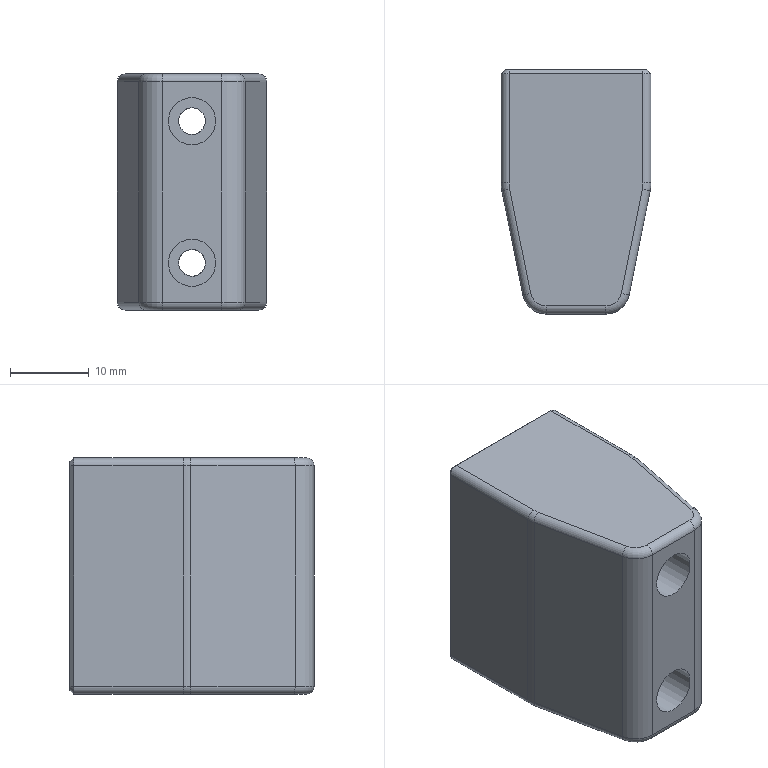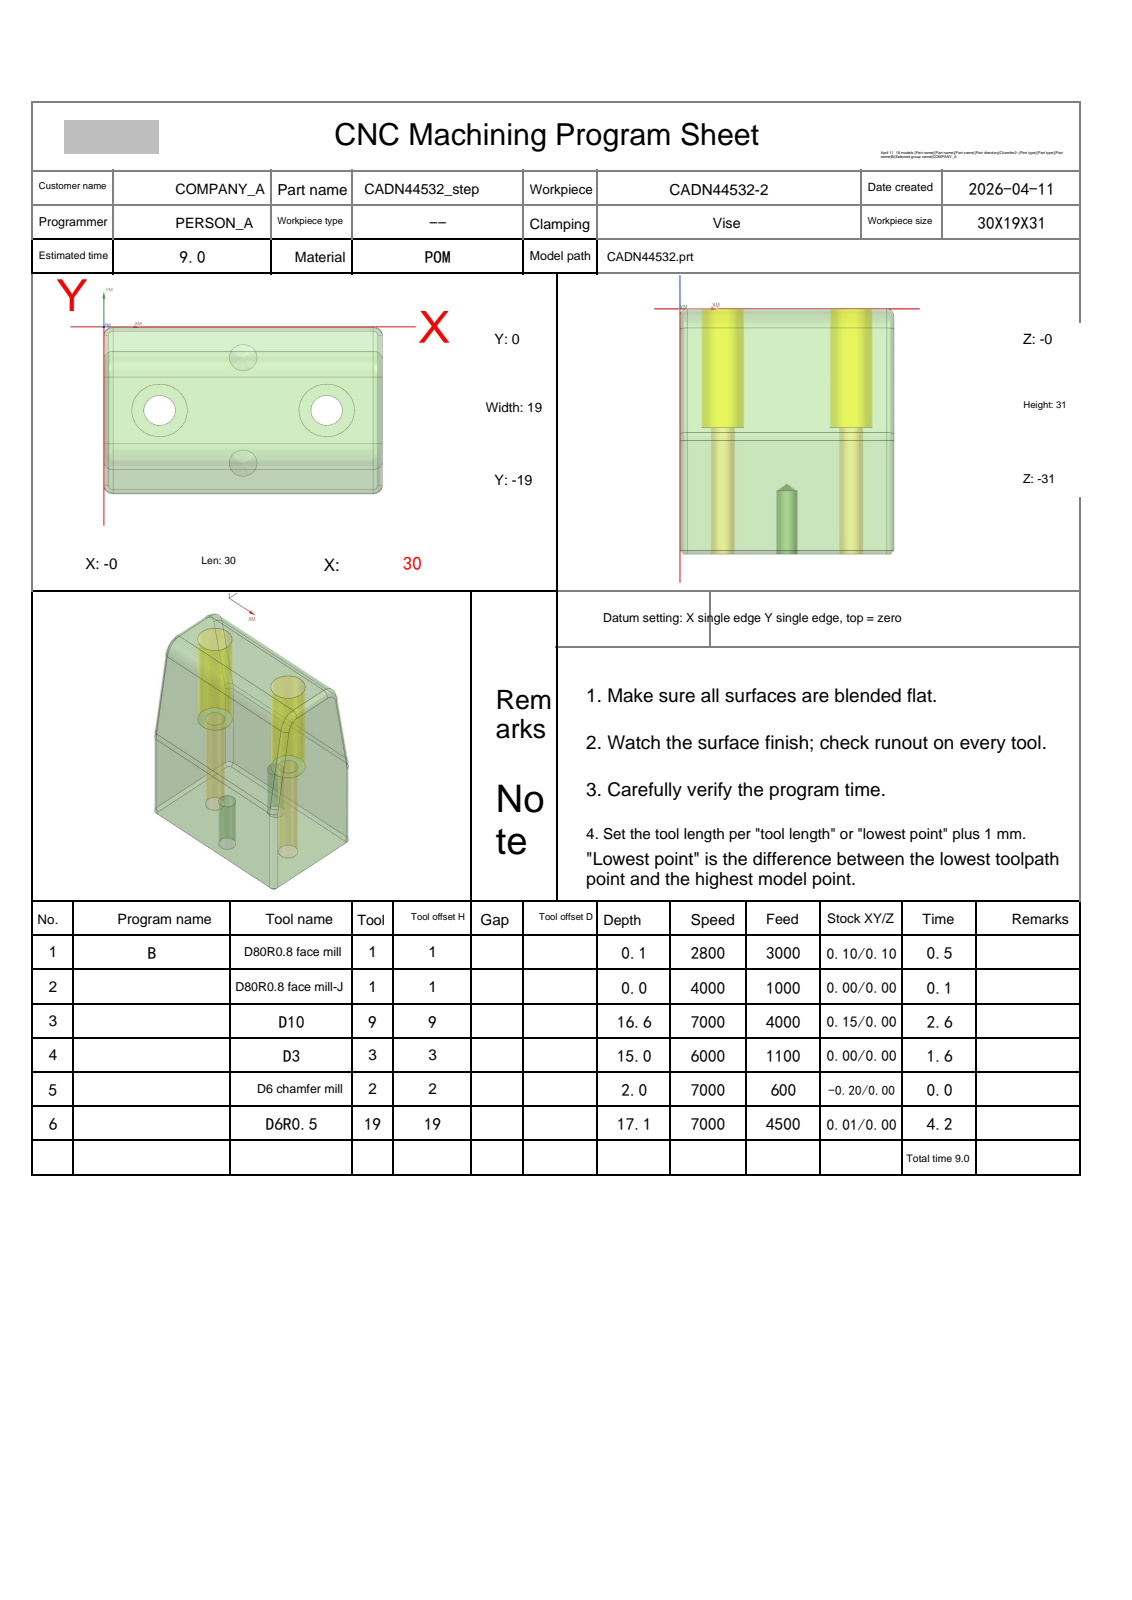NC program | NX | posted by the shop | part box 19 x 31 x 30 mm
Lines 1 to 2364 of 6576, first 1874 of 2362 lines:
%
O0001
(Machine time: 10.35 MIN)
(===Total Tool:5===)
(T1=D80R0.8 face mill D=80.  R=0.8  D-  H01 Z=-0.   )
(T9=D10     D=10.  R=0.   D-  H09 Z=-16.62)
(T3=D3      D=3.   R=0.   D-  H03 Z=-15.  )
(T2=D6 chamfer mill   D=6.   R=0.   D-  H02 Z=-2.   )
(T19=D6R0.5 D=6.   R=0.5  D-  H19 Z=-17.12)
G80 G90 G17 G49 G40
G91 G28 Z0
M01
N1 T01 M06
(D80R0.8 face mill  D=80. R=0.8 H=01 ce=0.10 di=0.10)
G00 G90 G54 X82.097 Y-9.5 M03 S2800
G43 H01 Z20.
M08
Z6.011
G01 Z4.011 F3000.
X70.097
X-40.097
X-52.097
Z6.011
G00 X82.097
Z5.522
G01 Z3.522
X70.097
X-40.097
X-52.097
Z5.522
G00 X82.097
Z5.033
G01 Z3.033
X70.097
X-40.097
X-52.097
Z5.033
G00 X82.097
Z4.544
G01 Z2.544
X70.097
X-40.097
X-52.097
Z4.544
G00 Z20.
X82.097
Z4.056
G01 Z2.056
X70.097
X-40.097
X-52.097
Z4.056
G00 Z20.
X82.097
Z3.567
G01 Z1.567
X70.097
X-40.097
X-52.097
Z3.567
G00 Z20.
X82.097
Z3.078
G01 Z1.078
X70.097
X-40.097
X-52.097
Z3.078
G00 Z20.
X82.097
Z2.589
G01 Z.589
X70.097
X-40.097
X-52.097
Z2.589
G00 Z20.
X82.097
Z2.1
G01 Z.1
X70.097
X-40.097
X-52.097
Z2.1
G00 Z20.
G91 G28 Z0.0
M05
M09
G91 G28 Z0.0
M01
N2 T01 M06
(D80R0.8 face mill-J  D=80. R=0.8 H=01 ce=0.00 di=0.00)
G00 G90 G54 X81.999 Y-9.499 M03 S4000
G43 H01 Z20.
M08
Z2.
G01 Z0.0 F1000.
X69.999
X-39.999 Y-9.501
X-51.999
Z2.
G00 Z20.
G91 G28 Z0.0
M05
M09
G91 G28 Z0.0
M01
N3 T09 M06
(D10  D=10. R=0. H=09 ce=0.15 di=0.00)
G00 G90 G54 X-9.322 Y-11.818 M03 S7000
G43 H09 Z14.8
M08
Z.485
G01 Z-.015 F4000.
G03 X-4.322 Y-6.818 I0.0 J5.
G02 X-4.345 Y-6.25 I7.038 J.568
X-3.6 Y-3.093 I7.061 J0.0
X.988 Y-.256 I4.589 J-2.293
G01 X29.008
G02 X34.224 Y-5.172 I0.0 J-5.226
G01 X34.322 Y-6.818
X34.386 Z-.028
X34.435 Z-.041
G03 X34.451 Y-6.237 I-10.057 J.581
X34.345 Y-4.78 I-10.074 J0.0
X29. Y-.059 I-5.478 J-.817
G01 X1.
G03 X-4.183 Y-4.095 I.106 J-5.481
X-4.461 Y-6.17 I7.588 J-2.075
X-4.435 Y-6.818 I7.867 J0.0
G01 X-4.495 Z-.061
X-4.546 Z-.082
G02 X-4.564 Y-6.232 I9.361 J.586
X-4.362 Y-4.298 I9.38 J0.0
X1. Y.139 I5.471 J-1.153
G01 X29.
G02 X34.456 Y-4.78 I-.127 J-5.626
X34.559 Y-6.281 I-10.952 J-1.502
X34.546 Y-6.818 I-11.055 J0.0
G01 X34.601 Z-.107
X34.648 Z-.133
G03 X34.668 Y-6.21 I-9.632 J.608
X34.44 Y-4.126 I-9.651 J0.0
X29. Y.328 I-5.548 J-1.227
G01 X1.
G03 X-4.44 Y-4.126 I.108 J-5.681
X-4.668 Y-6.21 I9.423 J-2.084
X-4.648 Y-6.818 I9.651 J0.0
G01 X-4.702 Z-.166
X-4.749 Z-.199
G02 X-4.768 Y-6.191 I10.301 J.627
X-4.555 Y-4.105 I10.32 J0.0
X1. Y.52 I5.679 J-1.172
G01 X29.
G02 X34.555 Y-4.105 I-.124 J-5.797
X34.768 Y-6.191 I-10.107 J-2.086
X34.749 Y-6.818 I-10.32 J0.0
G01 X34.798 Z-.239
X34.842 Z-.278
G03 X34.85 Y-6.302 I-17.25 J.516
X34.816 Y-5.229 I-17.258 J0.0
X33.856 Y-2.082 I-6.718 J-.329
X29. Y.706 I-4.938 J-2.978
G01 X1.
G03 X-1.935 Y-.14 I.091 J-5.828
X-4.71 Y-4.33 I3.349 J-5.231
X-4.855 Y-6.241 I12.477 J-1.911
X-4.842 Y-6.818 I12.622 J0.0
G01 X-4.886 Z-.323
X-4.925 Z-.368
G02 X-4.937 Y-6.246 I13.468 J.572
X-4.801 Y-4.33 I13.48 J0.0
X-3.372 Y-1.183 I6.49 J-1.049
X1. Y.885 I4.433 J-3.717
G01 X29.
G02 X34.193 Y-2.438 I-.084 J-5.851
X34.904 Y-5.229 I-6.578 J-3.16
X34.929 Y-6.37 I-25.428 J-1.14
X34.925 Y-6.818 I-25.453 J0.0
G01 X34.964 Z-.419
X34.998 Z-.47
G03 X35.009 Y-6.235 I-16.606 J.583
X34.949 Y-4.824 I-16.616 J0.0
X34.252 Y-2.321 I-6.99 J-.596
G01 X34.193 Y-2.201
X34.137 Y-2.082
G03 X29. Y1.057 I-5.219 J-2.767
G01 X1.
G03 X-3.742 Y-1.442 I.073 J-5.885
X-4.945 Y-4.78 I5.783 J-3.97
X-5.009 Y-6.235 I16.552 J-1.456
X-4.998 Y-6.818 I16.616 J0.0
G01 X-5.031 Z-.527
X-5.059 Z-.584
G02 X-5.067 Y-6.265 I19.985 J.553
X-5.012 Y-4.78 I19.992 J0.0
X-4.003 Y-1.633 I7.125 J-.549
X1. Y1.223 I5.064 J-3.062
G01 X29.
G02 X34.003 Y-1.633 I-.061 J-5.917
X35.012 Y-4.78 I-6.116 J-3.696
X35.067 Y-6.265 I-19.937 J-1.485
X35.059 Y-6.818 I-19.992 J0.0
G01 X35.085 Y-6.817 Z-.646
X35.107 Z-.708
G03 X35.111 Y-6.336 I-25.666 J.48
X35.064 Y-4.78 I-25.671 J0.0
X34.126 Y-1.633 I-7.287 J-.459
X29. Y1.381 I-5.186 J-2.955
G01 X1.
G03 X-4.126 Y-1.633 I.06 J-5.969
X-5.064 Y-4.78 I6.349 J-3.606
X-5.111 Y-6.336 I25.623 J-1.557
X-5.107 Y-6.817 I25.671 J0.0
G01 X-5.124 Z-.776
X-5.138 Z-.843
X-5.127 Y-5.229
G02 X-4.797 Y-2.981 I8.476 J-.093
X-2.137 Y.615 I6.1 J-1.73
X1. Y1.529 I3.219 J-5.206
G01 X29.
G02 X33.632 Y-.734 I-.05 J-5.974
G01 X33.672 Y-.785
G02 X34.894 Y-3.332 I-5.107 J-4.017
X35.127 Y-5.229 I-8.785 J-2.04
G01 X35.138 Y-6.817
X35.146 Z-.915
X35.15 Z-.987
X35.143 Y-5.229
G03 X35.049 Y-3.88 I-9.714 J-.001
X34.193 Y-1.373 I-6.723 J-.894
X29. Y1.669 I-5.248 J-3.008
G01 X1.
G03 X-4.336 Y-1.633 I.058 J-6.056
X-5.103 Y-4.33 I6.261 J-3.239
X-5.156 Y-6.188 I32.712 J-1.858
X-5.15 Y-6.817 I32.764 J0.0
G01 Y-6.81 Z-1.14
X-5.145 Y-4.78
G02 X-4.645 Y-2.127 I7.363 J-.014
X-1.935 Y1.019 I5.828 J-2.28
X1. Y1.798 I2.997 J-5.372
G01 X29.
G02 X33.885 Y-.734 I-.051 J-6.077
G01 X34.09 Y-1.051
G02 X34.965 Y-3.19 I-5.237 J-3.391
G01 X35.015 Y-3.431
G02 X35.145 Y-4.78 I-7.142 J-1.37
G01 X35.15 Y-6.81
Z-1.301
Y-4.78
X35.141 Y-4.33
G03 X34.264 Y-1.183 I-6.782 J-.194
X31.484 Y1.372 I-5.349 J-3.031
X29. Y1.917 I-2.573 J-5.79
G01 X1.
G03 X-.129 Y1.803 I.41 J-9.752
X-3.984 Y-.734 I1.17 J-5.975
X-5.141 Y-4.33 I5.59 J-3.782
G01 X-5.15 Y-4.78
Y-6.81
Z-1.47
Y-4.78
X-5.149 Y-4.33
G02 X-4.346 Y-1.183 I6.788 J-.057
X1. Y2.025 I5.395 J-2.932
G01 X29.
G02 X34.565 Y-1.633 I-.048 J-6.135
X35.149 Y-4.33 I-6.184 J-2.752
G01 X35.15 Y-4.78
Y-6.81
Z-1.645
Y-4.33
X35.151 Y-4.22
G03 X34.193 Y-.806 I-6.565 J0.0
X29. Y2.121 I-5.224 J-3.199
G01 X1.
G03 X-3.454 Y.166 I.025 J-6.106
X-5.139 Y-3.88 I4.699 J-4.331
G01 X-5.15 Y-4.33
Y-6.81
Z-1.827
Y-4.33
X-5.144 Y-3.88
G02 X-2.541 Y1.065 I6.296 J-.156
X1. Y2.205 I3.585 J-5.061
G01 X29.
G02 X33.544 Y.166 I-.042 J-6.175
X35.144 Y-3.88 I-4.754 J-4.219
G01 X35.15 Y-4.33
Y-6.81
Z-2.013
Y-4.33
X35.149 Y-3.941
G03 X34.812 Y-1.934 I-6.206 J-.012
G01 X34.708 Y-1.633
G03 X30.129 Y2.169 I-5.747 J-2.264
X29. Y2.278 I-1.412 J-8.736
G01 X1.
G03 X.302 Y2.227 I.283 J-8.845
X-2.387 Y1.248 I.673 J-6.029
X-5.149 Y-3.88 I3.499 J-5.193
G01 X-5.15 Y-4.33
Y-6.81
Z-2.204
Y-3.88
Y-3.866
G02 X-2.731 Y1.065 I6.235 J0.0
X1. Y2.337 I3.774 J-4.96
G01 X29.
G02 X32.731 Y1.065 I-.043 J-6.232
X35.15 Y-3.866 I-3.816 J-4.931
G01 Y-3.88
Y-6.81
Z-2.399
Y-3.88
X35.138 Y-3.431
G03 X29. Y2.384 I-6.159 J-.354
G01 X1.
G03 X-5.138 Y-3.431 I.021 J-6.169
G01 X-5.15 Y-3.88
Y-6.81
Z-2.594
Y-3.88
X-5.14 Y-3.431
G02 X1. Y2.423 I6.152 J-.305
G01 X29.
G02 X35.14 Y-3.431 I-.012 J-6.159
G01 X35.15 Y-3.88
Y-6.81
Z-2.79
Y-3.88
X35.143 Y-3.431
G03 X29. Y2.463 I-6.155 J-.268
G01 X1.
G03 X-5.143 Y-3.431 I.013 J-6.161
G01 X-5.15 Y-3.88
Y-6.81
Z-2.986
Y-3.88
X-5.144 Y-3.431
G02 X1. Y2.502 I6.157 J-.228
G01 X29.
G02 X35.144 Y-3.431 I-.013 J-6.161
G01 X35.15 Y-3.88
Y-6.81
Z-3.182
Y-3.88
X35.145 Y-3.431
G03 X29. Y2.542 I-6.159 J-.189
G01 X1.
G03 X-5.145 Y-3.431 I.013 J-6.162
G01 X-5.15 Y-3.88
Y-6.81
Z-3.378
Y-3.88
X-5.147 Y-3.431
G02 X1. Y2.581 I6.161 J-.15
G01 X29.
G02 X35.147 Y-3.431 I-.014 J-6.162
G01 X35.15 Y-3.88
Y-6.81
Z-3.575
Y-3.88
X35.148 Y-3.431
G03 X29. Y2.621 I-6.163 J-.113
G01 X1.
G03 X-5.148 Y-3.431 I.015 J-6.164
G01 X-5.15 Y-3.88
Y-6.81
Z-3.771
X-5.149 Y-3.431
G02 X1. Y2.66 I6.165 J-.075
G01 X29.
G02 X35.149 Y-3.431 I-.016 J-6.166
G01 X35.15 Y-6.81
Z-3.967
Y-3.431
G03 X29. Y2.7 I-6.166 J-.035
G01 X1.
G03 X-5.15 Y-3.431 I.016 J-6.166
G01 Y-6.81
Z-4.163
Y-3.431
Y-3.428
G02 X1. Y2.739 I6.167 J0.0
G01 X29.
G02 X35.15 Y-3.428 I-.017 J-6.167
G01 Y-3.431
Y-6.81
Z-4.359
Y-3.431
Y-3.39
G03 X29. Y2.779 I-6.169 J0.0
G01 X1.
G03 X-5.15 Y-3.39 I.019 J-6.169
G01 Y-3.431
Y-6.81
Z-4.555
Y-3.431
Y-3.364
G02 X-2.387 Y1.798 I6.204 J0.0
X1. Y2.818 I3.397 J-5.147
G01 X29.
G02 X35.012 Y-2.082 I-.007 J-6.147
X35.15 Y-3.377 I-5.993 J-1.294
G01 Y-3.431
Y-6.81
Z-4.751
Y-3.431
X35.136 Y-2.981
G03 X29. Y2.858 I-6.146 J-.315
G01 X1.
G03 X-3.332 Y1.065 I.006 J-6.145
X-5.151 Y-3.333 I4.408 J-4.397
G01 X-5.15 Y-3.431
Y-6.81
Z-4.947
Y-3.431
X-5.138 Y-2.981
G02 X1. Y2.897 I6.149 J-.277
G01 X29.
G02 X35.138 Y-2.981 I-.011 J-6.156
G01 X35.15 Y-3.431
Y-6.81
Z-5.143
Y-3.431
X35.14 Y-2.981
G03 X29. Y2.937 I-6.152 J-.238
G01 X1.
G03 X-5.14 Y-2.981 I.011 J-6.156
G01 X-5.15 Y-3.431
Y-6.81
Z-5.339
Y-3.431
X-5.142 Y-2.981
G02 X1. Y2.976 I6.157 J-.202
G01 X29.
G02 X35.142 Y-2.981 I-.015 J-6.16
G01 X35.15 Y-3.431
Y-6.81
Z-5.535
Y-3.189
G03 X34.957 Y-1.633 I-6.365 J0.0
X29. Y3.016 I-5.967 J-1.505
G01 X1.
G03 X-.58 Y2.809 I.045 J-6.474
X-5.144 Y-2.981 I1.605 J-5.959
G01 X-5.15 Y-3.431
Y-6.81
Z-5.731
Y-3.431
X-5.147 Y-2.981
G02 X-.58 Y2.848 I6.177 J-.135
X1. Y3.055 I1.625 J-6.264
G01 X29.
G02 X35.128 Y-2.638 I-.011 J-6.157
X35.15 Y-3.228 I-7.829 J-.59
G01 Y-6.81
Z-5.927
Y-3.431
X35.149 Y-3.086
G03 X34.979 Y-1.633 I-6.441 J-.019
X29. Y3.095 I-5.992 J-1.433
G01 X1.
G03 X-1.484 Y2.569 I.018 J-6.217
X-5.149 Y-2.981 I2.524 J-5.652
G01 X-5.15 Y-3.431
Y-6.81
Z-6.123
Y-2.981
G02 X1. Y3.135 I6.165 J-.05
G01 X29.
G02 X35.15 Y-2.981 I-.02 J-6.17
G01 Y-6.81
Z-6.319
Y-2.981
X35.129 Y-2.532
G03 X29. Y3.174 I-6.14 J-.451
G01 X1.
G03 X-5.15 Y-2.981 I.017 J-6.166
G01 Y-6.81
Z-6.515
Y-2.981
X-5.143 Y-2.757
G02 X1. Y3.214 I6.156 J-.188
G01 X29.
G02 X35.15 Y-2.956 I-.019 J-6.169
G01 Y-2.981
Y-6.81
Z-6.711
Y-2.981
X35.141 Y-2.686
G03 X29. Y3.253 I-6.152 J-.217
G01 X1.
G03 X-5.145 Y-2.757 I.014 J-6.161
G01 X-5.15 Y-2.981
Y-6.81
Z-6.907
Y-2.981
X-5.147 Y-2.757
G02 X-1.254 Y2.863 I6.178 J-.122
X1. Y3.293 I2.272 J-5.79
G01 X29.
G02 X35.143 Y-2.686 I-.013 J-6.159
G01 X35.15 Y-2.981
Y-6.81
Z-7.104
Y-2.981
X35.151 Y-2.884
G03 X34.92 Y-1.183 I-6.389 J0.0
X29. Y3.332 I-5.929 J-1.635
G01 X1.
G03 X-2.387 Y2.312 I.01 J-6.167
X-5.149 Y-2.757 I3.445 J-5.165
G01 X-5.15 Y-2.981
Y-6.81
Z-7.3
Y-2.757
X-5.148 Y-2.686
G02 X-2.387 Y2.352 I6.202 J-.123
X1. Y3.372 I3.398 J-5.149
G01 X29.
G02 X35.031 Y-1.633 I-.007 J-6.144
X35.15 Y-2.785 I-5.534 J-1.153
G01 Y-6.81
Z-7.496
Y-2.981
X35.149 Y-2.672
G03 X34.806 Y-.734 I-6.368 J-.128
X29. Y3.411 I-5.815 J-2.007
G01 X1.
G03 X-4.645 Y-.311 I.012 J-6.161
X-5.149 Y-2.672 I5.894 J-2.493
G01 X-5.15 Y-2.757
Y-6.81
Z-7.692
X-5.149 Y-2.644
X-5.144 Y-2.532
X-5.125 Y-2.195
G02 X-1.484 Y2.925 I6.166 J-.531
G01 X-1.032 Y3.102
X-.58 Y3.244
X-.289 Y3.312
X-.129 Y3.346
X.323 Y3.409
X.774 Y3.446
X1. Y3.451
X29.
G02 X34.942 Y-1.142 I-.01 J-6.153
X35.149 Y-2.749 I-6.136 J-1.608
G01 X35.15 Y-6.81
Z-7.888
Y-2.644
G03 X34.833 Y-.734 I-6.326 J-.068
X29. Y3.49 I-5.841 J-1.927
G01 X1.
G03 X-.58 Y3.283 I.046 J-6.477
X-5.146 Y-2.532 I1.609 J-5.963
G01 X-5.15 Y-2.644
Y-6.81
Z-8.084
Y-2.679
Y-2.64
G02 X-2.387 Y2.51 I6.204 J-.013
X1. Y3.53 I3.398 J-5.151
G01 X29.
G02 X34.846 Y-.734 I-.01 J-6.154
X35.15 Y-2.64 I-6. J-1.934
G01 Y-2.679
Y-6.81
Z-8.28
Y-2.679
Y-2.601
Y-2.6
G03 X29. Y3.569 I-6.169 J0.0
G01 X1.
G03 X-5.15 Y-2.6 I.019 J-6.169
G01 Y-2.601
Y-2.679
Y-6.81
Z-8.476
Y-2.679
Y-2.561
Y-2.557
G02 X1. Y3.609 I6.166 J0.0
G01 X29.
G02 X35.15 Y-2.557 I-.016 J-6.166
G01 Y-2.561
Y-2.679
Y-6.81
Z-8.672
Y-2.679
Y-2.522
Y-2.519
G03 X29. Y3.648 I-6.167 J0.0
G01 X1.
G03 X-5.15 Y-2.519 I.018 J-6.167
G01 Y-2.522
Y-2.679
Y-6.81
Z-8.868
Y-2.679
X-5.149 Y-2.482
Y-2.477
G02 X1. Y3.688 I6.165 J0.0
G01 X29.
G02 X35.149 Y-2.477 I-.016 J-6.165
G01 Y-2.482
X35.15 Y-2.679
Y-6.81
Z-9.064
Y-2.679
X35.149 Y-2.443
Y-2.441
G03 X29. Y3.727 I-6.168 J0.0
G01 X1.
G03 X-5.149 Y-2.441 I.02 J-6.168
G01 Y-2.443
X-5.15 Y-2.679
Y-6.81
Z-9.26
Y-2.679
X-5.149 Y-2.403
G02 X-2.203 Y2.863 I6.193 J-.008
X1. Y3.767 I3.212 J-5.253
G01 X29.
G02 X35.021 Y-1.183 I-.006 J-6.145
X35.149 Y-2.395 I-5.671 J-1.212
G01 Y-2.403
X35.15 Y-2.679
Y-6.81
Z-9.456
Y-2.679
Y-2.364
X35.139 Y-2.082
G03 X29. Y3.806 I-6.149 J-.266
G01 X1.
G03 X-2.387 Y2.787 I.011 J-6.169
X-5.15 Y-2.364 I3.445 J-5.164
G01 Y-2.679
Y-6.81
Z-9.652
Y-2.679
Y-2.324
G02 X-3.419 Y1.964 I6.222 J-.019
X1. Y3.846 I4.424 J-4.258
G01 X29.
G02 X35.141 Y-2.082 I-.011 J-6.156
G01 X35.15 Y-2.324
Y-2.679
Y-6.81
Z-9.848
Y-2.679
Y-2.285
G03 X34.949 Y-.734 I-6.426 J-.045
X29. Y3.886 I-5.957 J-1.532
G01 X1.
G03 X-3.457 Y1.964 I.006 J-6.144
X-5.15 Y-2.285 I4.532 J-4.267
G01 Y-2.679
Y-6.81
Z-10.044
Y-2.679
Y-2.245
G02 X-3.495 Y1.964 I6.226 J-.018
X1. Y3.925 I4.504 J-4.19
G01 X29.
G02 X34.96 Y-.734 I-.01 J-6.154
X35.15 Y-2.245 I-6.248 J-1.554
G01 Y-2.679
Y-6.81
Z-10.24
Y-2.679
Y-2.206
G03 X34.841 Y-.284 I-6.299 J-.027
X29. Y3.965 I-5.85 J-1.903
G01 X1.
G03 X-2.387 Y2.945 I.011 J-6.171
X-5.15 Y-2.206 I3.444 J-5.164
G01 Y-2.679
Y-6.81
Z-10.436
Y-2.679
Y-2.166
Y-2.162
G02 X1. Y4.004 I6.166 J0.0
G01 X29.
G02 X35.15 Y-2.162 I-.016 J-6.166
G01 Y-2.166
Y-2.679
Y-6.81
Z-10.633
Y-2.679
Y-2.126
Y-2.122
G03 X29. Y4.044 I-6.166 J0.0
G01 X1.
G03 X-5.15 Y-2.122 I.016 J-6.166
G01 Y-2.126
Y-2.679
Y-6.81
Z-10.829
Y-2.679
Y-2.103
Y-2.086
G02 X1. Y4.083 I6.169 J0.0
G01 X29.
G02 X35.15 Y-2.086 I-.019 J-6.169
G01 Y-2.103
Y-2.679
Y-6.81
Z-11.025
Y-2.679
Y-2.103
Y-2.047
G03 X29. Y4.123 I-6.17 J0.0
G01 X1.
G03 X-5.15 Y-2.047 I.02 J-6.17
G01 Y-2.103
Y-2.679
Y-6.81
Z-11.221
Y-2.679
Y-2.103
X-5.151 Y-2.021
G02 X-2.387 Y3.142 I6.206 J0.0
X1. Y4.162 I3.397 J-5.148
G01 X29.
G02 X34.901 Y-.284 I-.009 J-6.151
X35.15 Y-2.05 I-6.136 J-1.766
G01 Y-2.103
Y-2.679
Y-6.81
Z-11.417
Y-2.679
Y-2.103
X35.151 Y-2.021
G03 X34.912 Y-.284 I-6.44 J0.0
X29. Y4.202 I-5.92 J-1.664
G01 X1.
G03 X-3.328 Y2.413 I.006 J-6.145
X-5.151 Y-1.992 I4.412 J-4.406
G01 X-5.15 Y-2.103
Y-2.679
Y-6.81
Z-11.613
Y-2.679
Y-2.103
X-5.151 Y-1.972
G02 X-4.599 Y.615 I6.332 J0.0
X1. Y4.241 I5.606 J-2.52
G01 X29.
G02 X34.923 Y-.284 I-.009 J-6.15
X35.151 Y-1.992 I-6.279 J-1.708
G01 X35.15 Y-2.103
Y-2.679
Y-6.81
Z-11.809
Y-2.679
Y-2.103
X35.152 Y-1.963
G03 X34.934 Y-.284 I-6.583 J0.0
X29. Y4.281 I-5.942 J-1.585
G01 X1.
G03 X-4.618 Y.615 I.01 J-6.152
X-5.152 Y-1.945 I5.866 J-2.56
G01 X-5.15 Y-2.103
Y-2.679
Y-6.81
Z-12.005
Y-2.679
Y-2.103
X-5.152 Y-1.937
G02 X-4.871 Y-.015 I6.704 J0.0
X1. Y4.32 I5.882 J-1.823
G01 X29.
G02 X34.945 Y-.284 I-.009 J-6.151
X35.152 Y-1.935 I-6.461 J-1.651
G01 X35.15 Y-2.103
Y-2.679
Y-6.81
Z-12.201
Y-2.679
Y-2.103
X35.153 Y-1.906
G03 X34.955 Y-.284 I-6.764 J0.0
X29. Y4.36 I-5.965 J-1.51
G01 X1.
G03 X-4.823 Y.166 I.01 J-6.152
X-5.153 Y-1.893 I6.237 J-2.058
X-5.15 Y-2.103 I6.568 J0.0
G01 Y-2.679
Y-6.81
Z-12.397
Y-2.679
Y-2.103
G02 X-5.155 Y-1.861 I6.601 J.243
X-4.836 Y.166 I6.605 J0.0
X1. Y4.399 I5.845 J-1.918
G01 X29.
G02 X34.966 Y-.284 I-.011 J-6.156
X35.154 Y-1.878 I-6.684 J-1.594
X35.15 Y-2.103 I-6.871 J0.0
G01 Y-2.679
Y-6.81
Z-12.593
Y-2.679
Y-2.103
G03 X35.154 Y-1.854 I-7.036 J.249
X34.977 Y-.284 I-7.04 J0.0
X29. Y4.439 I-5.99 J-1.437
G01 X1.
G03 X-4.849 Y.166 I.011 J-6.155
X-5.156 Y-1.832 I6.365 J-1.998
X-5.15 Y-2.103 I6.671 J0.0
G01 Y-2.679
Y-6.81
Z-12.789
Y-2.679
Y-2.103
G02 X-5.153 Y-1.874 I8.753 J.23
X-5.096 Y-.879 I8.756 J0.0
X1. Y4.478 I6.111 J-.807
G01 X29.
G02 X35.126 Y-1.183 I-.012 J-6.158
X35.153 Y-1.88 I-9.108 J-.697
X35.15 Y-2.103 I-9.134 J0.0
G01 Y-2.679
Y-6.81
Z-12.985
Y-2.679
Y-2.103
G03 X35.153 Y-1.873 I-9.748 J.23
X35.128 Y-1.183 I-9.751 J0.0
X29. Y4.518 I-6.14 J-.456
G01 X1.
G03 X-5.128 Y-1.183 I.012 J-6.157
X-5.153 Y-1.873 I9.726 J-.69
X-5.15 Y-2.103 I9.751 J0.0
G01 Y-2.679
Y-6.81
Z-13.181
Y-2.679
Y-2.103
G02 X-5.153 Y-1.87 I10.669 J.233
X-5.131 Y-1.183 I10.671 J0.0
X1. Y4.558 I6.141 J-.414
G01 X29.
G02 X35.131 Y-1.183 I-.011 J-6.155
X35.153 Y-1.87 I-10.649 J-.687
X35.15 Y-2.103 I-10.671 J0.0
G01 Y-2.679
Y-6.81
Z-13.377
Y-2.679
Y-2.103
G03 X35.152 Y-1.87 I-11.985 J.233
X35.133 Y-1.183 I-11.988 J0.0
X29. Y4.597 I-6.143 J-.374
G01 X1.
G03 X-5.133 Y-1.183 I.01 J-6.154
X-5.152 Y-1.87 I11.968 J-.687
X-5.15 Y-2.103 I11.988 J0.0
G01 Y-2.679
Y-6.81
Z-13.573
Y-2.679
Y-2.103
G02 X-5.152 Y-1.87 I13.674 J.233
X-5.135 Y-1.183 I13.676 J0.0
X1. Y4.637 I6.145 J-.335
G01 X29.
G02 X35.135 Y-1.183 I-.009 J-6.153
X35.152 Y-1.87 I-13.659 J-.687
X35.15 Y-2.103 I-13.676 J0.0
G01 Y-2.679
Y-6.81
Z-13.769
Y-2.679
Y-2.103
G03 X35.152 Y-1.871 I-15.918 J.233
X35.137 Y-1.183 I-15.919 J0.0
X29. Y4.676 I-6.147 J-.295
G01 X1.
G03 X-5.137 Y-1.183 I.01 J-6.154
X-5.152 Y-1.871 I15.904 J-.688
X-5.15 Y-2.103 I15.919 J0.0
G01 Y-2.679
Y-6.81
Z-13.965
Y-2.679
Y-2.103
G02 X-5.152 Y-1.871 I19.044 J.232
X-5.139 Y-1.183 I19.045 J0.0
X1. Y4.716 I6.15 J-.256
G01 X29.
G02 X35.139 Y-1.183 I-.011 J-6.155
X35.152 Y-1.871 I-19.033 J-.688
X35.15 Y-2.103 I-19.045 J0.0
G01 Y-2.679
Y-6.81
Z-14.162
Y-2.679
Y-2.103
G03 X35.153 Y-1.808 I-13.747 J.295
X35.111 Y-.734 I-13.75 J0.0
G01 X35.096 Y-.602
X34.944 Y.166
X34.92 Y.252
G03 X29. Y4.755 I-5.931 J-1.655
G01 X1.
G03 X-5.141 Y-1.183 I.012 J-6.158
G01 X-5.15 Y-2.103
Y-2.679
Y-6.81
Z-14.358
Y-2.679
Y-2.103
X-5.143 Y-1.183
G02 X1. Y4.795 I6.16 J-.185
G01 X29.
G02 X35.143 Y-1.183 I-.017 J-6.163
G01 X35.15 Y-2.103
Y-2.679
Y-6.81
Z-14.554
Y-2.679
Y-2.103
X35.146 Y-1.302
X35.145 Y-1.217
G03 X29. Y4.834 I-6.156 J-.107
G01 X1.
G03 X-.58 Y4.627 I.047 J-6.488
X-5.146 Y-1.183 I1.608 J-5.962
G01 X-5.15 Y-2.103
Y-2.679
Y-6.81
Z-14.75
Y-2.679
Y-2.103
X-5.148 Y-1.183
G02 X-1.484 Y4.348 I6.185 J-.118
X1. Y4.874 I2.501 J-5.686
G01 X29.
G02 X34.902 Y.434 I-.011 J-6.157
X35.148 Y-1.289 I-6.027 J-1.74
G01 X35.15 Y-2.103
Y-2.679
Y-6.81
Z-14.946
Y-2.679
Y-2.103
X35.149 Y-1.183
G03 X29. Y4.913 I-6.165 J-.069
G01 X1.
G03 X-5.149 Y-1.183 I.015 J-6.165
G01 X-5.15 Y-2.103
Y-2.679
Y-6.81
Z-15.142
Y-2.679
Y-2.103
G02 X-5.157 Y-1.651 I15.188 J.453
X-5.129 Y-.734 I15.195 J0.0
X1. Y4.953 I6.14 J-.472
G01 X29.
G02 X35.129 Y-.734 I-.011 J-6.159
X35.154 Y-1.727 I-20.172 J-.994
X35.15 Y-2.103 I-20.196 J0.0
G01 Y-2.679
Y-6.81
Z-15.338
Y-2.679
Y-2.103
G03 X35.153 Y-1.724 I-23.121 J.379
X35.132 Y-.734 I-23.124 J0.0
X29. Y4.992 I-6.143 J-.433
G01 X1.
G03 X-5.132 Y-.734 I.011 J-6.159
X-5.156 Y-1.647 I17.249 J-.913
X-5.15 Y-2.103 I17.273 J0.0
G01 Y-2.679
Y-6.81
Z-15.534
Y-2.679
Y-2.103
G02 X-5.155 Y-1.647 I20.095 J.457
X-5.135 Y-.734 I20.1 J0.0
X1. Y5.032 I6.146 J-.394
G01 X29.
G02 X35.135 Y-.734 I-.012 J-6.159
X35.153 Y-1.725 I-26.918 J-.991
X35.15 Y-2.103 I-26.937 J0.0
G01 Y-2.679
Y-6.81
Z-15.73
Y-2.679
Y-2.103
Y-1.183
X35.151 Y-1.099
G03 X29. Y5.07 I-6.169 J0.0
G01 X1.
G03 X-5.151 Y-1.099 I.019 J-6.169
G01 X-5.15 Y-1.183
Y-2.103
Y-2.679
Y-6.81
Z-15.928
Y-2.679
Y-2.103
G02 X-5.154 Y-1.648 I30.423 J.456
X-5.14 Y-.734 I30.426 J0.0
X1. Y5.102 I6.153 J-.326
G01 X29.
G02 X35.14 Y-.734 I-.013 J-6.162
X35.152 Y-1.727 I-40.909 J-.993
X35.15 Y-2.103 I-40.921 J0.0
G01 Y-2.679
Y-6.81
Z-16.101
Y-2.679
Y-2.103
G03 X35.152 Y-1.728 I-46.124 J.376
X35.141 Y-.734 I-46.126 J0.0
X29. Y5.123 I-6.153 J-.304
G01 X1.
G03 X-5.141 Y-.734 I.012 J-6.16
X-5.153 Y-1.648 I34.233 J-.914
X-5.15 Y-2.103 I34.245 J0.0
G01 Y-2.679
Y-6.81
Z-16.273
Y-2.679
Y-2.103
G02 X-5.153 Y-1.648 I39.158 J.455
X-5.145 Y-.888 I39.161 J0.0
X-.434 Y4.96 I6.133 J-.119
X1. Y5.138 I1.518 J-6.374
G01 X29.
G02 X30.449 Y4.957 I-.085 J-6.552
X35.145 Y-.91 I-1.436 J-5.962
X35.152 Y-1.728 I-52.841 J-.818
X35.15 Y-2.103 I-52.847 J0.0
G01 Y-2.679
Y-6.81
Z-16.446
Y-2.679
Y-2.103
X35.143 Y-.734
G03 X31.032 Y4.795 I-6.145 J-.277
X29. Y5.147 I-2.1 J-6.085
G01 X1.
G03 X.261 Y5.095 I.175 J-7.693
X-5.144 Y-.964 I.728 J-6.09
G01 X-5.15 Y-2.103
Y-2.679
Y-6.81
Z-16.619
Y-2.679
Y-2.103
X-5.144 Y-.734
X-5.102 Y-.231
X-5.096 Y-.19
G02 X-5.016 Y.279 I6.096 J-.81
X1. Y5.149 I6.017 J-1.281
G01 X29.
G02 X35.016 Y.275 I-.001 J-6.152
X35.096 Y-.19 I-6.016 J-1.275
X35.15 Y-1.026 I-6.495 J-.837
G01 Y-2.103
Y-2.679
Y-6.81
G00 Z14.8
X39.322 Y-7.182
Z.485
G01 Z-.015
G03 X34.322 Y-12.182 I0.0 J-5.
G02 X34.345 Y-12.75 I-7.038 J-.568
X33.6 Y-15.907 I-7.061 J0.0
X29.012 Y-18.744 I-4.589 J2.293
G01 X.992
G02 X-4.224 Y-13.828 I0.0 J5.226
G01 X-4.322 Y-12.182
X-4.386 Z-.028
X-4.435 Z-.041
G03 X-4.451 Y-12.763 I10.057 J-.581
X-4.345 Y-14.22 I10.074 J0.0
X1. Y-18.941 I5.478 J.817
G01 X29.
G03 X34.183 Y-14.905 I-.106 J5.481
X34.461 Y-12.83 I-7.588 J2.075
X34.435 Y-12.182 I-7.867 J0.0
G01 X34.495 Z-.061
X34.546 Z-.082
G02 X34.564 Y-12.768 I-9.361 J-.586
X34.362 Y-14.702 I-9.38 J0.0
X29. Y-19.139 I-5.471 J1.153
G01 X1.
G02 X-4.456 Y-14.22 I.127 J5.626
X-4.559 Y-12.719 I10.952 J1.502
X-4.546 Y-12.182 I11.055 J0.0
G01 X-4.601 Z-.107
X-4.648 Z-.133
G03 X-4.668 Y-12.79 I9.632 J-.608
X-4.44 Y-14.874 I9.651 J0.0
X1. Y-19.328 I5.548 J1.227
G01 X29.
G03 X34.44 Y-14.874 I-.108 J5.681
X34.668 Y-12.79 I-9.423 J2.084
X34.648 Y-12.182 I-9.651 J0.0
G01 X34.702 Z-.166
X34.749 Z-.199
G02 X34.768 Y-12.809 I-10.301 J-.627
X34.555 Y-14.895 I-10.32 J0.0
X29. Y-19.52 I-5.679 J1.172
G01 X1.
G02 X-4.555 Y-14.895 I.124 J5.797
X-4.768 Y-12.809 I10.107 J2.086
X-4.749 Y-12.182 I10.32 J0.0
G01 X-4.798 Z-.239
X-4.842 Z-.278
G03 X-4.85 Y-12.698 I17.25 J-.516
X-4.816 Y-13.771 I17.258 J0.0
X-3.856 Y-16.918 I6.718 J.329
X1. Y-19.706 I4.938 J2.978
G01 X29.
G03 X31.935 Y-18.86 I-.091 J5.828
X34.71 Y-14.67 I-3.349 J5.231
X34.855 Y-12.759 I-12.477 J1.911
X34.842 Y-12.182 I-12.622 J0.0
G01 X34.886 Z-.323
X34.925 Z-.368
G02 X34.937 Y-12.754 I-13.468 J-.572
X34.801 Y-14.67 I-13.48 J0.0
X33.372 Y-17.817 I-6.49 J1.049
X29. Y-19.885 I-4.433 J3.717
G01 X1.
G02 X-4.193 Y-16.562 I.084 J5.851
X-4.904 Y-13.771 I6.578 J3.16
X-4.929 Y-12.63 I25.428 J1.14
X-4.925 Y-12.182 I25.453 J0.0
G01 X-4.964 Z-.419
X-4.998 Z-.47
G03 X-5.009 Y-12.765 I16.606 J-.583
X-4.949 Y-14.176 I16.616 J0.0
X-4.252 Y-16.679 I6.99 J.596
G01 X-4.193 Y-16.799
X-4.137 Y-16.918
G03 X1. Y-20.057 I5.219 J2.767
G01 X29.
G03 X33.742 Y-17.558 I-.073 J5.885
X34.945 Y-14.22 I-5.783 J3.97
X35.009 Y-12.765 I-16.552 J1.456
X34.998 Y-12.182 I-16.616 J0.0
G01 X35.031 Z-.527
X35.059 Z-.584
G02 X35.067 Y-12.735 I-19.985 J-.553
X35.012 Y-14.22 I-19.992 J0.0
X34.003 Y-17.367 I-7.125 J.549
X29. Y-20.223 I-5.064 J3.062
G01 X1.
G02 X-4.003 Y-17.367 I.061 J5.917
X-5.012 Y-14.22 I6.116 J3.696
X-5.067 Y-12.735 I19.937 J1.485
X-5.059 Y-12.182 I19.992 J0.0
G01 X-5.085 Y-12.183 Z-.646
X-5.107 Z-.708
G03 X-5.111 Y-12.664 I25.666 J-.48
X-5.064 Y-14.22 I25.671 J0.0
X-4.126 Y-17.367 I7.287 J.459
X1. Y-20.381 I5.186 J2.955
G01 X29.
G03 X34.126 Y-17.367 I-.06 J5.969
X35.064 Y-14.22 I-6.349 J3.606
X35.111 Y-12.664 I-25.623 J1.557
X35.107 Y-12.183 I-25.671 J0.0
G01 X35.124 Z-.776
X35.138 Z-.843
X35.127 Y-13.771
G02 X34.797 Y-16.019 I-8.476 J.093
X32.137 Y-19.615 I-6.1 J1.73
X29. Y-20.529 I-3.219 J5.206
G01 X1.
G02 X-3.632 Y-18.266 I.05 J5.974
G01 X-3.672 Y-18.215
G02 X-4.894 Y-15.668 I5.107 J4.017
X-5.127 Y-13.771 I8.785 J2.04
G01 X-5.138 Y-12.183
X-5.146 Z-.915
X-5.15 Z-.987
X-5.143 Y-13.771
G03 X-5.049 Y-15.12 I9.714 J.001
X-4.193 Y-17.627 I6.723 J.894
X1. Y-20.669 I5.248 J3.008
G01 X29.
G03 X34.336 Y-17.367 I-.058 J6.056
X35.103 Y-14.67 I-6.261 J3.239
X35.156 Y-12.812 I-32.712 J1.858
X35.15 Y-12.183 I-32.764 J0.0
G01 Y-12.19 Z-1.14
X35.145 Y-14.22
G02 X34.645 Y-16.873 I-7.363 J.014
X31.935 Y-20.019 I-5.828 J2.28
X29. Y-20.798 I-2.997 J5.372
G01 X1.
G02 X-3.885 Y-18.266 I.051 J6.077
G01 X-4.09 Y-17.949
G02 X-4.965 Y-15.81 I5.237 J3.391
G01 X-5.015 Y-15.569
G02 X-5.145 Y-14.22 I7.142 J1.37
G01 X-5.15 Y-12.19
Z-1.301
Y-14.22
X-5.141 Y-14.67
G03 X-4.264 Y-17.817 I6.782 J.194
X-1.484 Y-20.372 I5.349 J3.031
X1. Y-20.917 I2.573 J5.79
G01 X29.
G03 X30.129 Y-20.803 I-.41 J9.752
X33.984 Y-18.266 I-1.17 J5.975
X35.141 Y-14.67 I-5.59 J3.782
G01 X35.15 Y-14.22
Y-12.19
Z-1.47
Y-14.22
X35.149 Y-14.67
G02 X34.346 Y-17.817 I-6.788 J.057
X29. Y-21.025 I-5.395 J2.932
G01 X1.
G02 X-4.565 Y-17.367 I.048 J6.135
X-5.149 Y-14.67 I6.184 J2.752
G01 X-5.15 Y-14.22
Y-12.19
Z-1.645
Y-14.67
X-5.151 Y-14.78
G03 X-4.193 Y-18.194 I6.565 J0.0
X1. Y-21.121 I5.224 J3.199
G01 X29.
G03 X33.454 Y-19.166 I-.025 J6.106
X35.139 Y-15.12 I-4.699 J4.331
G01 X35.15 Y-14.67
Y-12.19
Z-1.827
Y-14.67
X35.144 Y-15.12
G02 X32.541 Y-20.065 I-6.296 J.156
X29. Y-21.205 I-3.585 J5.061
G01 X1.
G02 X-3.544 Y-19.166 I.042 J6.175
X-5.144 Y-15.12 I4.754 J4.219
G01 X-5.15 Y-14.67
Y-12.19
Z-2.013
Y-14.67
X-5.149 Y-15.059
G03 X-4.812 Y-17.066 I6.206 J.012
G01 X-4.708 Y-17.367
G03 X-.129 Y-21.169 I5.747 J2.264
X1. Y-21.278 I1.412 J8.736
G01 X29.
G03 X29.698 Y-21.227 I-.283 J8.845
X32.387 Y-20.248 I-.673 J6.029
X35.149 Y-15.12 I-3.499 J5.193
G01 X35.15 Y-14.67
Y-12.19
Z-2.204
Y-15.12
Y-15.134
G02 X32.731 Y-20.065 I-6.235 J0.0
X29. Y-21.337 I-3.774 J4.96
G01 X1.
G02 X-2.731 Y-20.065 I.043 J6.232
X-5.15 Y-15.134 I3.816 J4.931
G01 Y-15.12
Y-12.19
Z-2.399
Y-15.12
X-5.138 Y-15.569
G03 X1. Y-21.384 I6.159 J.354
G01 X29.
G03 X35.138 Y-15.569 I-.021 J6.169
G01 X35.15 Y-15.12
Y-12.19
Z-2.594
Y-15.12
X35.14 Y-15.569
G02 X29. Y-21.423 I-6.152 J.305
G01 X1.
G02 X-5.14 Y-15.569 I.012 J6.159
G01 X-5.15 Y-15.12
Y-12.19
Z-2.79
Y-15.12
X-5.143 Y-15.569
G03 X1. Y-21.463 I6.155 J.268
G01 X29.
G03 X35.143 Y-15.569 I-.013 J6.161
G01 X35.15 Y-15.12
Y-12.19
Z-2.986
Y-15.12
X35.144 Y-15.569
G02 X29. Y-21.502 I-6.157 J.228
G01 X1.
G02 X-5.144 Y-15.569 I.013 J6.161
G01 X-5.15 Y-15.12
Y-12.19
Z-3.182
Y-15.12
X-5.145 Y-15.569
G03 X1. Y-21.542 I6.159 J.189
G01 X29.
G03 X35.145 Y-15.569 I-.013 J6.162
G01 X35.15 Y-15.12
Y-12.19
Z-3.378
Y-15.12
X35.147 Y-15.569
G02 X29. Y-21.581 I-6.161 J.15
G01 X1.
G02 X-5.147 Y-15.569 I.014 J6.162
G01 X-5.15 Y-15.12
Y-12.19
Z-3.575
Y-15.12
X-5.148 Y-15.569
G03 X1. Y-21.621 I6.163 J.113
G01 X29.
G03 X35.148 Y-15.569 I-.015 J6.164
G01 X35.15 Y-15.12
Y-12.19
Z-3.771
X35.149 Y-15.569
G02 X29. Y-21.66 I-6.165 J.075
G01 X1.
G02 X-5.149 Y-15.569 I.016 J6.166
G01 X-5.15 Y-12.19
Z-3.967
Y-15.569
G03 X1. Y-21.7 I6.166 J.035
G01 X29.
G03 X35.15 Y-15.569 I-.016 J6.166
G01 Y-12.19
Z-4.163
Y-15.569
Y-15.572
G02 X29. Y-21.739 I-6.167 J0.0
G01 X1.
G02 X-5.15 Y-15.572 I.017 J6.167
G01 Y-15.569
Y-12.19
Z-4.359
Y-15.569
Y-15.61
G03 X1. Y-21.779 I6.169 J0.0
G01 X29.
G03 X35.15 Y-15.61 I-.019 J6.169
G01 Y-15.569
Y-12.19
Z-4.555
Y-15.569
Y-15.636
G02 X32.387 Y-20.798 I-6.204 J0.0
X29. Y-21.818 I-3.397 J5.147
G01 X1.
G02 X-5.012 Y-16.918 I.007 J6.147
X-5.15 Y-15.629 I5.938 J1.289
G01 Y-15.569
Y-12.19
Z-4.751
Y-15.569
X-5.136 Y-16.019
G03 X1. Y-21.858 I6.146 J.315
G01 X29.
G03 X33.332 Y-20.065 I-.006 J6.145
X35.151 Y-15.667 I-4.408 J4.397
G01 X35.15 Y-15.569
Y-12.19
Z-4.947
Y-15.569
X35.138 Y-16.019
G02 X29. Y-21.897 I-6.149 J.277
G01 X1.
G02 X-4.924 Y-17.367 I.008 J6.15
X-5.151 Y-15.67 I6.24 J1.697
G01 X-5.15 Y-15.569
Y-12.19
Z-5.143
Y-15.569
X-5.14 Y-16.019
G03 X1. Y-21.937 I6.152 J.238
G01 X29.
G03 X35.14 Y-16.019 I-.011 J6.156
G01 X35.15 Y-15.569
Y-12.19
Z-5.339
Y-15.569
X35.142 Y-16.019
G02 X29. Y-21.976 I-6.157 J.202
G01 X1.
G02 X-5.142 Y-16.019 I.015 J6.16
G01 X-5.15 Y-15.569
Y-12.19
Z-5.535
Y-15.811
G03 X-4.957 Y-17.367 I6.365 J0.0
X1. Y-22.016 I5.967 J1.505
G01 X29.
G03 X30.58 Y-21.809 I-.045 J6.474
X35.144 Y-16.019 I-1.605 J5.959
G01 X35.15 Y-15.569
Y-12.19
Z-5.731
Y-15.569
X35.147 Y-16.019
G02 X30.58 Y-21.848 I-6.177 J.135
X29. Y-22.055 I-1.625 J6.264
G01 X1.
G02 X-5.128 Y-16.362 I.011 J6.157
X-5.15 Y-15.772 I7.829 J.59
G01 Y-12.19
Z-5.927
Y-15.569
X-5.149 Y-15.914
G03 X-4.979 Y-17.367 I6.441 J.019
X1. Y-22.095 I5.992 J1.433
G01 X29.
G03 X31.484 Y-21.569 I-.018 J6.217
X35.149 Y-16.019 I-2.524 J5.652
G01 X35.15 Y-15.569
Y-12.19
Z-6.123
Y-16.019
G02 X29. Y-22.135 I-6.169 J.054
G01 X1.
G02 X-5.15 Y-16.019 I.016 J6.165
G01 Y-12.19
Z-6.319
Y-16.019
G03 X1. Y-22.174 I6.166 J.011
G01 X29.
G03 X30.58 Y-21.967 I-.043 J6.459
X35.15 Y-16.019 I-1.608 J5.965
G01 Y-12.19
Z-6.515
Y-16.019
Y-16.044
G02 X29. Y-22.214 I-6.169 J0.0
G01 X1.
G02 X-5.15 Y-16.046 I.017 J6.167
G01 Y-16.019
Y-12.19
Z-6.711
Y-16.019
X-5.145 Y-16.243
G03 X1. Y-22.253 I6.159 J.151
G01 X29.
G03 X35.141 Y-16.314 I-.011 J6.156
G01 X35.15 Y-16.019
Y-12.19
Z-6.907
Y-16.019
X35.143 Y-16.314
G02 X29. Y-22.293 I-6.156 J.18
G01 X1.
G02 X-5.017 Y-17.367 I.006 J6.145
X-5.15 Y-16.15 I5.495 J1.218
G01 Y-12.19
Z-7.104
Y-16.019
X-5.151 Y-16.12
G03 X-4.92 Y-17.817 I6.353 J0.0
X1. Y-22.332 I5.929 J1.635
G01 X29.
G03 X30.58 Y-22.125 I-.043 J6.46
X35.146 Y-16.314 I-1.606 J5.961
G01 X35.15 Y-16.019
Y-12.19
Z-7.3
Y-16.019
X35.148 Y-16.314
G02 X32.387 Y-21.352 I-6.202 J.123
X29. Y-22.372 I-3.398 J5.149
G01 X1.
G02 X-5.031 Y-17.367 I.007 J6.144
X-5.15 Y-16.243 I5.462 J1.144
G01 Y-12.19
Z-7.496
Y-16.243
G03 X-4.806 Y-18.266 I6.351 J.04
X1. Y-22.411 I5.815 J2.007
G01 X29.
G03 X34.645 Y-18.69 I-.012 J6.161
X35.15 Y-16.207 I-5.847 J2.483
G01 Y-12.19
Z-7.692
X35.149 Y-16.356
X35.144 Y-16.468
X35.125 Y-16.805
G02 X31.484 Y-21.925 I-6.166 J.531
G01 X31.032 Y-22.102
X30.58 Y-22.244
X30.289 Y-22.312
X30.129 Y-22.346
X29.677 Y-22.409
X29.226 Y-22.446
X29. Y-22.451
X1.
G02 X-4.953 Y-17.817 I.01 J6.153
X-5.15 Y-16.243 I6.239 J1.581
G01 Y-12.19
Z-7.888
Y-16.356
G03 X-4.833 Y-18.266 I6.326 J.068
X1. Y-22.49 I5.841 J1.927
G01 X29.
G03 X30.58 Y-22.283 I-.046 J6.477
X35.146 Y-16.468 I-1.609 J5.963
G01 X35.15 Y-16.356
Y-12.19
Z-8.084
Y-16.321
Y-16.36
G02 X32.387 Y-21.51 I-6.204 J.013
X29. Y-22.53 I-3.398 J5.151
G01 X1.
G02 X-4.846 Y-18.266 I.01 J6.154
X-5.15 Y-16.36 I6. J1.934
G01 Y-16.321
Y-12.19
Z-8.28
Y-16.321
Y-16.399
Y-16.401
G03 X1. Y-22.569 I6.169 J0.0
G01 X29.
G03 X35.15 Y-16.401 I-.019 J6.169
G01 Y-16.399
Y-16.321
Y-12.19
Z-8.476
Y-16.321
Y-16.439
Y-16.443
G02 X29. Y-22.609 I-6.166 J0.0
G01 X1.
G02 X-5.15 Y-16.443 I.016 J6.166
G01 Y-16.439
Y-16.321
Y-12.19
Z-8.672
Y-16.321
Y-16.478
Y-16.482
G03 X1. Y-22.648 I6.166 J0.0
G01 X29.
G03 X35.15 Y-16.481 I-.018 J6.167
G01 Y-16.478
Y-16.321
Y-12.19
Z-8.868
Y-16.321
X35.149 Y-16.518
Y-16.523
G02 X29. Y-22.688 I-6.165 J0.0
G01 X1.
G02 X-5.149 Y-16.523 I.016 J6.165
G01 Y-16.518
X-5.15 Y-16.321
Y-12.19
Z-9.064
Y-16.321
X-5.149 Y-16.557
Y-16.559
G03 X1. Y-22.727 I6.168 J0.0
G01 X29.
G03 X35.149 Y-16.559 I-.02 J6.168
G01 Y-16.557
X35.15 Y-16.321
Y-12.19
Z-9.26
Y-16.321
X35.149 Y-16.597
G02 X32.203 Y-21.863 I-6.193 J.008
X29. Y-22.767 I-3.212 J5.253
G01 X1.
G02 X-5.021 Y-17.817 I.006 J6.145
X-5.149 Y-16.605 I5.671 J1.212
G01 Y-16.597
X-5.15 Y-16.321
Y-12.19
Z-9.456
Y-16.321
Y-16.636
X-5.139 Y-16.918
G03 X1. Y-22.806 I6.149 J.266
G01 X29.
G03 X32.387 Y-21.787 I-.011 J6.169
X35.15 Y-16.636 I-3.445 J5.164
G01 Y-16.321
Y-12.19
Z-9.652
Y-16.321
Y-16.676
G02 X33.419 Y-20.964 I-6.222 J.019
X29. Y-22.846 I-4.424 J4.258
G01 X1.
G02 X-5.141 Y-16.918 I.011 J6.156
G01 X-5.15 Y-16.676
Y-16.321
Y-12.19
Z-9.848
Y-16.321
Y-16.715
G03 X-4.949 Y-18.266 I6.426 J.045
X1. Y-22.886 I5.957 J1.532
G01 X29.
G03 X33.457 Y-20.964 I-.006 J6.144
X35.15 Y-16.715 I-4.532 J4.267
G01 Y-16.321
Y-12.19
Z-10.044
Y-16.321
Y-16.755
G02 X33.495 Y-20.964 I-6.226 J.018
X29. Y-22.925 I-4.504 J4.19
G01 X1.
G02 X-4.96 Y-18.266 I.01 J6.154
X-5.15 Y-16.755 I6.248 J1.554
G01 Y-16.321
Y-12.19
Z-10.24
Y-16.321
Y-16.794
G03 X-4.841 Y-18.716 I6.299 J.027
X1. Y-22.965 I5.85 J1.903
G01 X29.
G03 X32.387 Y-21.945 I-.011 J6.171
X35.15 Y-16.794 I-3.444 J5.164
G01 Y-16.321
Y-12.19
Z-10.436
Y-16.321
Y-16.834
Y-16.838
G02 X29. Y-23.004 I-6.166 J0.0
G01 X1.
G02 X-5.15 Y-16.838 I.016 J6.166
G01 Y-16.834
Y-16.321
Y-12.19
Z-10.633
Y-16.321
Y-16.874
Y-16.878
G03 X1. Y-23.044 I6.166 J0.0
G01 X29.
G03 X35.15 Y-16.878 I-.016 J6.166
G01 Y-16.874
Y-16.321
Y-12.19
Z-10.829
Y-16.321
Y-16.897
Y-16.914
G02 X29. Y-23.083 I-6.169 J0.0
G01 X1.
G02 X-5.15 Y-16.914 I.019 J6.169
G01 Y-16.897
Y-16.321
Y-12.19
Z-11.025
Y-16.321
Y-16.897
Y-16.953
G03 X1. Y-23.123 I6.17 J0.0
G01 X29.
G03 X35.15 Y-16.953 I-.02 J6.17
G01 Y-16.897
Y-16.321
Y-12.19
Z-11.221
Y-16.321
Y-16.897
X35.151 Y-16.979
G02 X32.387 Y-22.142 I-6.206 J0.0
X29. Y-23.162 I-3.397 J5.148
G01 X1.
G02 X-4.901 Y-18.716 I.009 J6.151
X-5.15 Y-16.95 I6.136 J1.766
G01 Y-16.897
Y-16.321
Y-12.19
Z-11.417
Y-16.321
Y-16.897
X-5.151 Y-16.979
G03 X-4.912 Y-18.716 I6.44 J0.0
X1. Y-23.202 I5.92 J1.664
G01 X29.
G03 X33.328 Y-21.413 I-.006 J6.145
X35.151 Y-17.008 I-4.412 J4.406
G01 X35.15 Y-16.897
Y-16.321
Y-12.19
Z-11.613
Y-16.321
Y-16.897
X35.151 Y-17.028
G02 X34.599 Y-19.615 I-6.332 J0.0
X29. Y-23.241 I-5.606 J2.52
G01 X1.
G02 X-4.923 Y-18.716 I.009 J6.15
X-5.151 Y-17.008 I6.279 J1.708
G01 X-5.15 Y-16.897
Y-16.321
Y-12.19
Z-11.809
Y-16.321
Y-16.897
X-5.152 Y-17.037
G03 X-4.934 Y-18.716 I6.583 J0.0
X1. Y-23.281 I5.942 J1.585
G01 X29.
G03 X34.618 Y-19.615 I-.01 J6.152
X35.152 Y-17.055 I-5.866 J2.56
G01 X35.15 Y-16.897
Y-16.321
Y-12.19
Z-12.005
Y-16.321
Y-16.897
X35.152 Y-17.063
G02 X34.871 Y-18.985 I-6.704 J0.0
X29. Y-23.32 I-5.882 J1.823
G01 X1.
G02 X-4.945 Y-18.716 I.009 J6.151
X-5.152 Y-17.065 I6.461 J1.651
G01 X-5.15 Y-16.897
Y-16.321
Y-12.19
Z-12.201
Y-16.321
Y-16.897
X-5.153 Y-17.094
G03 X-4.955 Y-18.716 I6.764 J0.0
X1. Y-23.36 I5.965 J1.51
G01 X29.
G03 X34.823 Y-19.166 I-.01 J6.152
X35.153 Y-17.107 I-6.237 J2.058
X35.15 Y-16.897 I-6.568 J0.0
G01 Y-16.321
Y-12.19
Z-12.397
Y-16.321
Y-16.897
G02 X35.155 Y-17.139 I-6.601 J-.243
X34.836 Y-19.166 I-6.605 J0.0
X29. Y-23.399 I-5.845 J1.918
G01 X1.
G02 X-4.966 Y-18.716 I.011 J6.156
X-5.154 Y-17.122 I6.684 J1.594
X-5.15 Y-16.897 I6.871 J0.0
G01 Y-16.321
Y-12.19
Z-12.593
Y-16.321
Y-16.897
G03 X-5.154 Y-17.146 I7.036 J-.249
X-4.977 Y-18.716 I7.04 J0.0
X1. Y-23.439 I5.99 J1.437
G01 X29.
G03 X34.849 Y-19.166 I-.011 J6.155
X35.156 Y-17.168 I-6.365 J1.998
X35.15 Y-16.897 I-6.671 J0.0
G01 Y-16.321
Y-12.19
Z-12.789
Y-16.321
Y-16.897
G02 X35.153 Y-17.126 I-8.753 J-.23
X35.096 Y-18.121 I-8.756 J0.0
X29. Y-23.478 I-6.111 J.807
G01 X1.
G02 X-5.126 Y-17.817 I.012 J6.158
X-5.153 Y-17.12 I9.108 J.697
X-5.15 Y-16.897 I9.134 J0.0
G01 Y-16.321
Y-12.19
Z-12.985
Y-16.321
Y-16.897
G03 X-5.153 Y-17.127 I9.748 J-.23
X-5.128 Y-17.817 I9.751 J0.0
X1. Y-23.518 I6.14 J.456
G01 X29.
G03 X35.128 Y-17.817 I-.012 J6.157
X35.153 Y-17.127 I-9.726 J.69
X35.15 Y-16.897 I-9.751 J0.0
G01 Y-16.321
Y-12.19
Z-13.181
Y-16.321
Y-16.897
G02 X35.153 Y-17.13 I-10.669 J-.233
X35.131 Y-17.817 I-10.671 J0.0
X29. Y-23.558 I-6.141 J.415
G01 X1.
G02 X-5.131 Y-17.817 I.01 J6.155
X-5.153 Y-17.13 I10.649 J.687
X-5.15 Y-16.897 I10.671 J0.0
G01 Y-16.321
Y-12.19
Z-13.377
Y-16.321
Y-16.897
G03 X-5.152 Y-17.13 I11.985 J-.233
X-5.133 Y-17.817 I11.988 J0.0
X1. Y-23.597 I6.143 J.374
G01 X29.
G03 X35.133 Y-17.817 I-.01 J6.154
X35.152 Y-17.13 I-11.968 J.687
X35.15 Y-16.897 I-11.988 J0.0
G01 Y-16.321
Y-12.19
Z-13.573
Y-16.321
Y-16.897
G02 X35.152 Y-17.13 I-13.674 J-.233
X35.135 Y-17.817 I-13.676 J0.0
X29. Y-23.637 I-6.144 J.334
G01 X1.
G02 X-4.91 Y-19.166 I.01 J6.155
X-5.096 Y-18.279 I6.277 J1.785
X-5.153 Y-17.158 I11.045 J1.121
X-5.15 Y-16.897 I11.102 J0.0
G01 Y-16.321
Y-12.19
Z-13.769
Y-16.321
Y-16.897
G03 X-5.152 Y-17.129 I15.918 J-.233
X-5.137 Y-17.817 I15.919 J0.0
X1. Y-23.676 I6.147 J.295
G01 X29.
G03 X35.137 Y-17.817 I-.01 J6.154
X35.152 Y-17.129 I-15.904 J.688
X35.15 Y-16.897 I-15.919 J0.0
G01 Y-16.321
Y-12.19
Z-13.965
Y-16.321
Y-16.897
G02 X35.152 Y-17.129 I-19.044 J-.232
X35.139 Y-17.817 I-19.045 J0.0
X29. Y-23.716 I-6.15 J.256
G01 X1.
G02 X-5.139 Y-17.817 I.011 J6.155
X-5.152 Y-17.129 I19.033 J.688
X-5.15 Y-16.897 I19.045 J0.0
G01 Y-16.321
Y-12.19
Z-14.162
Y-16.321
Y-16.897
X-5.141 Y-17.817
G03 X1. Y-23.755 I6.154 J.219
G01 X29.
G03 X35.141 Y-17.817 I-.012 J6.158
G01 X35.15 Y-16.897
Y-16.321
Y-12.19